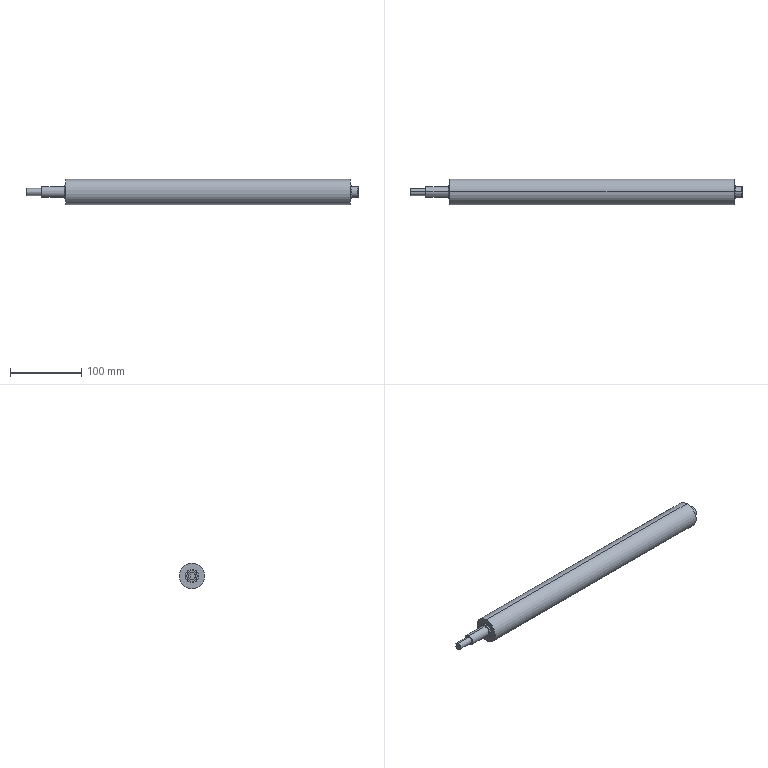Part | STEP file | PN_0015 | 1 solid | 39 faces | box 467 x 36 x 36 mm | volume 417063 mm3 | cone 15 | cylinder 14 | plane 10 | commonest cylinder face diameters 15 x4 19 x4 4 x2 10 x2 36 x2